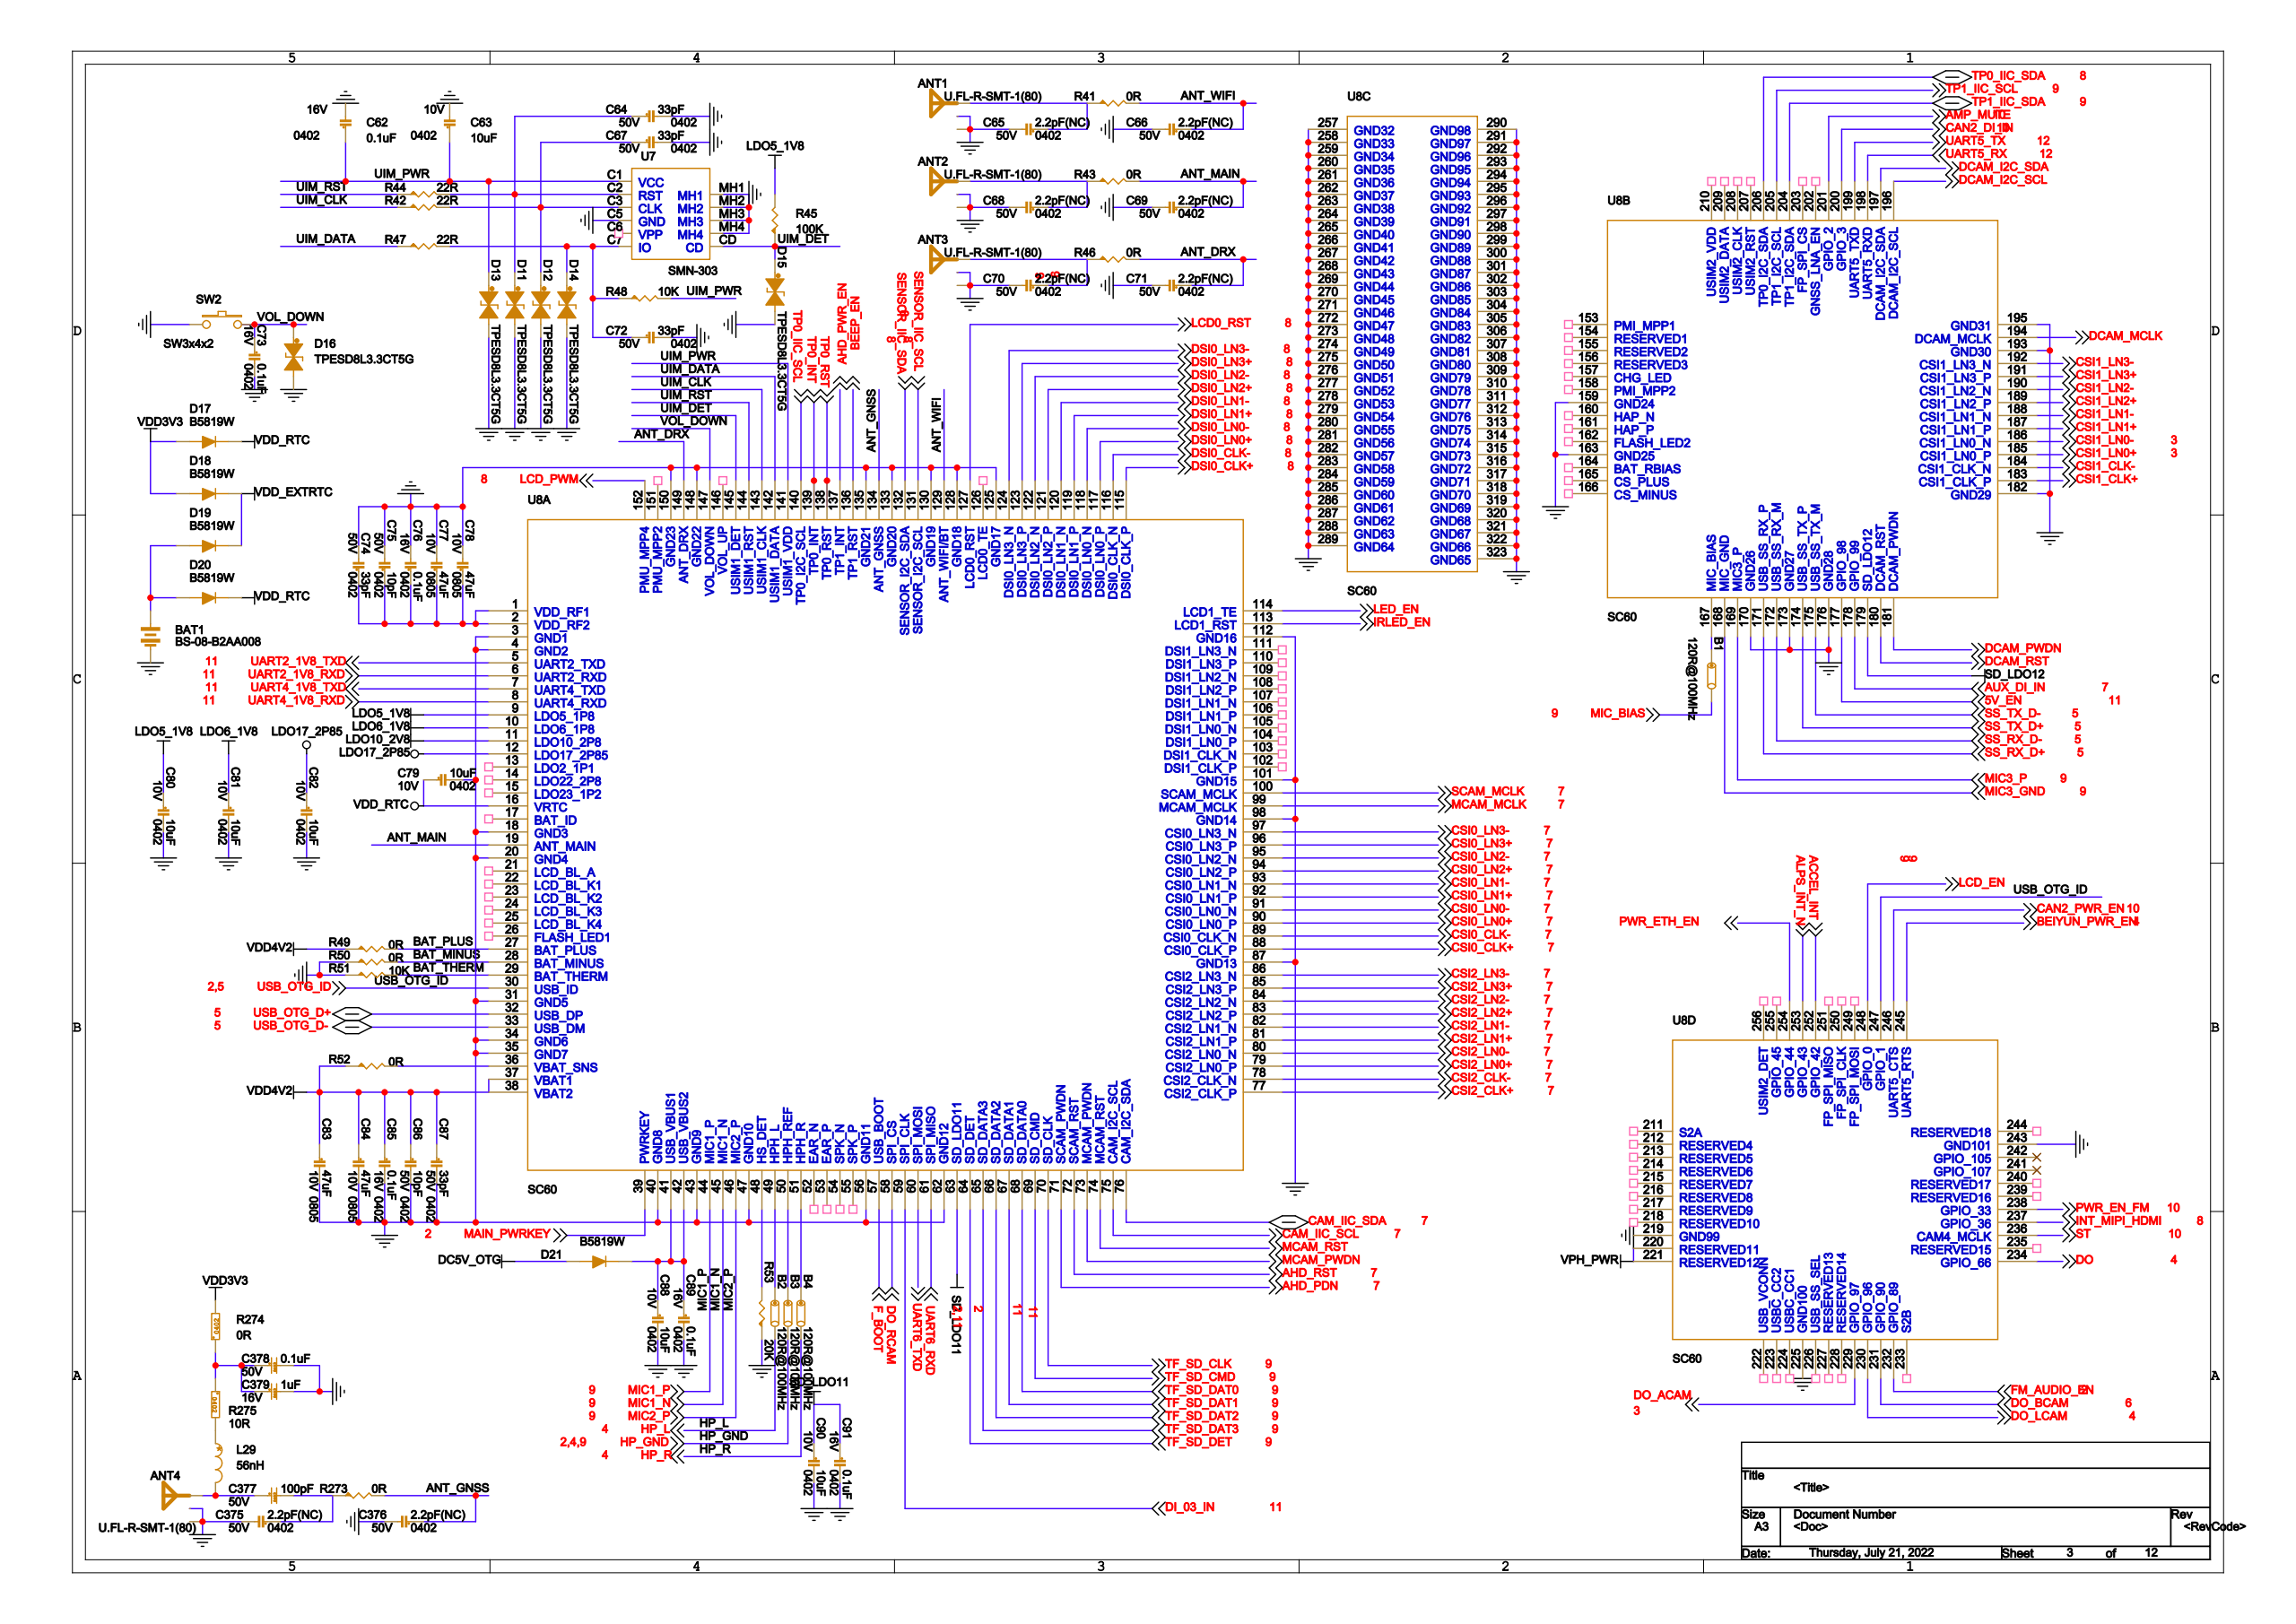Circuit board | Cadence Allegro | 970 parts | 627 nets | one sheet of the schematic
Parts on this sheet (reference | value | footprint):
ANT1 | U.FL-R-SMT-1(80) | IPEX
ANT2 | U.FL-R-SMT-1(80) | IPEX
ANT3 | U.FL-R-SMT-1(80) | IPEX
ANT4 | U.FL-R-SMT-1(80) | IPEX
B1 | 120R@100MHz | R0402
B2 | 120R@100MHz | R0402
B3 | 120R@100MHz | R0402
B4 | 120R@100MHz | R0402
BAT1 | BS-08-B2AA008 | CR2032
C62 | 0.1uF | C0402
C63 | 10uF | C0402
C64 | 33pF | C0402
C65 | 2.2pF(NC) | C0402
C66 | 2.2pF(NC) | C0402
C67 | 33pF | C0402
C68 | 2.2pF(NC) | C0402
C69 | 2.2pF(NC) | C0402
C70 | 2.2pF(NC) | C0402
C71 | 2.2pF(NC) | C0402
C72 | 33pF | C0402
C73 | 0.1uF | C0402
C74 | 33pF | C0402
C75 | 10pF | C0402
C76 | 0.1uF | C0402
C77 | 47uF | C0805
C78 | 47uF | C0805
C79 | 10uF | C0402
C80 | 10uF | C0402
C81 | 10uF | C0402
C82 | 10uF | C0402
C83 | 47uF | C0805
C84 | 47uF | C0805
C85 | 0.1uF | C0402
C86 | 10pF | C0402
C87 | 33pF | C0402
C88 | 10uF | C0402
C89 | 0.1uF | C0402
C90 | 10uF | C0402
C91 | 0.1uF | C0402
C375 | 2.2pF(NC) | C0402
C376 | 2.2pF(NC) | C0402
C377 | 100pF | C0402
C378 | 0.1uF | C0402
C379 | 1uF | C0402
D11 | TPESD8L3.3CT5G | DFN1006_2L
D12 | TPESD8L3.3CT5G | DFN1006_2L
D13 | TPESD8L3.3CT5G | DFN1006_2L
D14 | TPESD8L3.3CT5G | DFN1006_2L
D15 | TPESD8L3.3CT5G | DFN1006_2L
D16 | TPESD8L3.3CT5G | DFN1006_2L
D17 | B5819W | SOD-123
D18 | B5819W | SOD-123
D19 | B5819W | SOD-123
D20 | B5819W | SOD-123
D21 | B5819W | SOD-123
L29 | 56nH | R0402
R41 | 0R | R0402
R42 | 22R | R0402
R43 | 0R | R0402
R44 | 22R | R0402
R45 | 100K | R0402
R46 | 0R | R0402
R47 | 22R | R0402
R48 | 10K | R0402
R49 | 0R | R0402
R50 | 0R | R0402
R51 | 10K | R0402
R52 | 0R | R0402
R53 | 20K | R0402
R273 | 0R | R0402
R274 | 0R | R0402
R275 | 10R | R0402
SW2 | SW3x4x2 | SW3X4X2
U7 | SMN-303 | MICRO_SIM_SMN_303
U8 | SC60 | SC60
Nets of these parts (net: part-pin ...):
TP0_IIC_SCL: U8-140
VDD3V3: D17-1 D18-1 R274-2
GND: ANT1-2 ANT1-3 ANT2-2 ANT2-3 ANT3-2 ANT3-3 ANT4-2 ANT4-3 BAT1-2 C62-2 C63-2 C64-2 C65-2 C66-2 C67-2 C68-2 C69-2 C70-2 C71-2 C72-2 C73-2 C74-2 C75-2 C76-2 C77-2 C78-2 C79-2 C80-2 C81-2 C82-2 C83-2 C84-2 C85-2 C86-2 C87-2 C88-2 C89-2 C90-2 C91-2 C375-2 C376-2 C378-2 C379-2 D11-1 D12-1 D13-1 D14-1 D15-1 D16-1 R50-1 R51-1 R53-1 SW2-1 U7-C5 U7-MH1 U7-MH2 U7-MH3 U7-MH4 U8-3 U8-4 U8-18 U8-20 U8-31 U8-34 U8-35 U8-40 U8-43 U8-47 U8-56 U8-62 U8-87 U8-98 U8-101 U8-112 U8-125 U8-128 U8-130 U8-133 U8-135 U8-148 U8-150 U8-159 U8-163 U8-170 U8-173 U8-176 U8-182 U8-193 U8-195 U8-219 U8-225 U8-243 U8-257 U8-258 U8-259 U8-260 U8-261 U8-262 U8-263 U8-264 U8-265 U8-266 U8-267 U8-268 U8-269 U8-270 U8-271 U8-272 U8-273 U8-274 U8-275 U8-276 U8-277 U8-278 U8-279 U8-280 U8-281 U8-282 U8-283 U8-284 U8-285 U8-286 U8-287 U8-288 U8-289 U8-290 U8-291 U8-292 U8-293 U8-294 U8-295 U8-296 U8-297 U8-298 U8-299 U8-300 U8-301 U8-302 U8-303 U8-304 U8-305 U8-306 U8-307 U8-308 U8-309 U8-310 U8-311 U8-312 U8-313 U8-314 U8-315 U8-316 U8-317 U8-318 U8-319 U8-320 U8-321 U8-322 U8-323
INT_MIPI_HDMI: U8-237
LCD0_RST: U8-127
TP0_IIC_SDA: U8-206
VDD4V2: C83-1 C84-1 C85-1 C86-1 C87-1 R49-1 R52-1 U8-37 U8-38
LDO6_1V8: C81-1 U8-10
LCD_PWM: U8-152
MIC1_P: U8-44
MIC1_N: U8-45
MIC3_GND: U8-168
MIC3_P: U8-169
SENSOR_IIC_SCL: U8-131
SENSOR_IIC_SDA: U8-132
LDO10_2V8: U8-11
MCAM_RST: U8-74
CSI0_LN0+: U8-90
CSI0_LN0-: U8-91
CSI0_LN1+: U8-92
CSI0_LN1-: U8-93
CSI0_CLK+: U8-88
CSI0_CLK-: U8-89
MCAM_PWDN: U8-73
CSI0_LN2+: U8-94
CSI0_LN2-: U8-95
DCAM_RST: U8-180
DCAM_PWDN: U8-181
DCAM_I2C_SCL: U8-196
DCAM_I2C_SDA: U8-197
MCAM_MCLK: U8-99
CSI1_LN0-: U8-186
CSI1_LN1+: U8-187
CSI1_LN1-: U8-188
CSI1_CLK+: U8-183
CSI1_LN2+: U8-189
CSI1_LN2-: U8-190
N19662170: ANT4-1 C377-1 L29-2
N19662172: C375-1 C377-2 R273-1
N19663545: C378-1 C379-1 R274-1 R275-1
N196634830: L29-1 R275-2
LDO5_1V8: C80-1 R45-2 U8-9
USB_OTG_ID: U8-30 U8-247
CAM_IIC_SCL: U8-75
CAM_IIC_SDA: U8-76
DCAM_MCLK: U8-194
ALPS_INT_N: U8-253
MIC_BIAS: B1-2
VPH_PWR: U8-220 U8-221
VDD_EXTRTC: D18-2 D19-2
AHD_PDN: U8-71
DSI0_LN0+: U8-117
DSI0_LN0-: U8-118
DSI0_LN1+: U8-119
DSI0_LN1-: U8-120
DSI0_CLK+: U8-115
DSI0_CLK-: U8-116
DSI0_LN2+: U8-121
DSI0_LN2-: U8-122
DSI0_LN3+: U8-123
DSI0_LN3-: U8-124
IRLED_EN: U8-113
LED_EN: U8-114
LCD_EN: U8-248
CSI2_CLK-: U8-78
CSI2_CLK+: U8-77
CSI2_LN0-: U8-80
CSI2_LN1-: U8-82
CSI2_LN2-: U8-84
CSI2_LN3-: U8-86
CSI2_LN0+: U8-79
CSI2_LN1+: U8-81
CSI2_LN2+: U8-83
CSI2_LN3+: U8-85
N19376406: ANT1-1 C65-1 R41-1
N19375824: ANT2-1 C68-1 R43-1
N19376109: ANT3-1 C70-1 R46-1
N19231813: B1-1 U8-167
N19211601: B2-1 U8-49
HP_L: B2-2
N19211630: B3-1 U8-50
HP_GND: B3-2
N19211633: B4-1 U8-51
HP_R: B4-2
N19309091: BAT1-1 D19-1 D20-1
N19204544: C74-1 C75-1 C76-1 C77-1 C78-1 U8-1 U8-2
N19355924: C64-1 D11-2 R44-2 U7-C2
N19355913: C67-1 D12-2 R42-2 U7-C3
N19355903: C72-1 D14-2 R47-2 R48-1 U7-C7
ANT_GNSS: C376-1 R273-2 U8-134
ANT_WIFI: C66-1 R41-2 U8-129
ANT_MAIN: C69-1 R43-2 U8-19
ANT_DRX: C71-1 R46-2 U8-149
UIM_PWR: C62-1 C63-1 D13-2 R48-2 U7-C1 U8-141
UIM_DET: D15-2 R45-1 U7-CD U8-145
VOL_DOWN: C73-1 D16-2 SW2-2 U8-147
SD_LDO11: C90-1 C91-1 U8-63
DI_03_IN: U8-59
F_BOOT: U8-57
VDD_RTC: C79-1 D17-2 D20-2 U8-16
DC5V_OTG: D21-1
N19210596: C88-1 C89-1 D21-2 U8-41 U8-42
AUX_DI_IN: U8-178
BAT_PLUS: R49-2 U8-27
BAT_MINUS: R50-2 U8-28
N19208323: R52-2 U8-36
5V_EN: U8-177
PWR_EN_FM: U8-238
AHD_RST: U8-72
TF_SD_DAT0: U8-68
TF_SD_DAT1: U8-67
TF_SD_DAT2: U8-66
TF_SD_DAT3: U8-65
TF_SD_CLK: U8-70
TF_SD_CMD: U8-69
TF_SD_DET: U8-64
MAIN_PWRKEY: U8-39
UIM_CLK: R42-1 U8-143
UIM_RST: R44-1 U8-144
UIM_DATA: R47-1 U8-142
N19211098: R53-2 U8-48
PWR_ETH_EN: U8-254
AHD_PWR_EN: U8-137
BEEP_EN: U8-136
SD_LDO12: U8-179
DO_ACAM: U8-229
DO_LCAM: U8-230
DO_BCAM: U8-231
DO_RCAM: U8-58
CAN2_PWR_EN: U8-246
BAT_THERM: R51-2 U8-29
AMP_MUTE: U8-201
SCAM_MCLK: U8-100
UART6_RXD: U8-61
TP0_INT: U8-139
TP0_RST: U8-138
TP1_IIC_SCL: U8-205
TP1_IIC_SDA: U8-204
DO: U8-234
ST: U8-236
UART4_1V8_TXD: U8-7
UART4_1V8_RXD: U8-8
UART5_TX: U8-199
UART5_RX: U8-198
UART2_1V8_TXD: U8-5
UART2_1V8_RXD: U8-6
UART6_TXD: U8-60
USB_OTG_D+: U8-32
ACCEL_INT: U8-252
CSI0_LN3-: U8-97
CSI0_LN3+: U8-96
LDO17_2P85: C82-1 U8-12
MIC2_P: U8-46
CSI1_LN3-: U8-192
CSI1_LN3+: U8-191
SS_RX_D-: U8-172
SS_RX_D+: U8-171
SS_TX_D-: U8-175
SS_TX_D+: U8-174